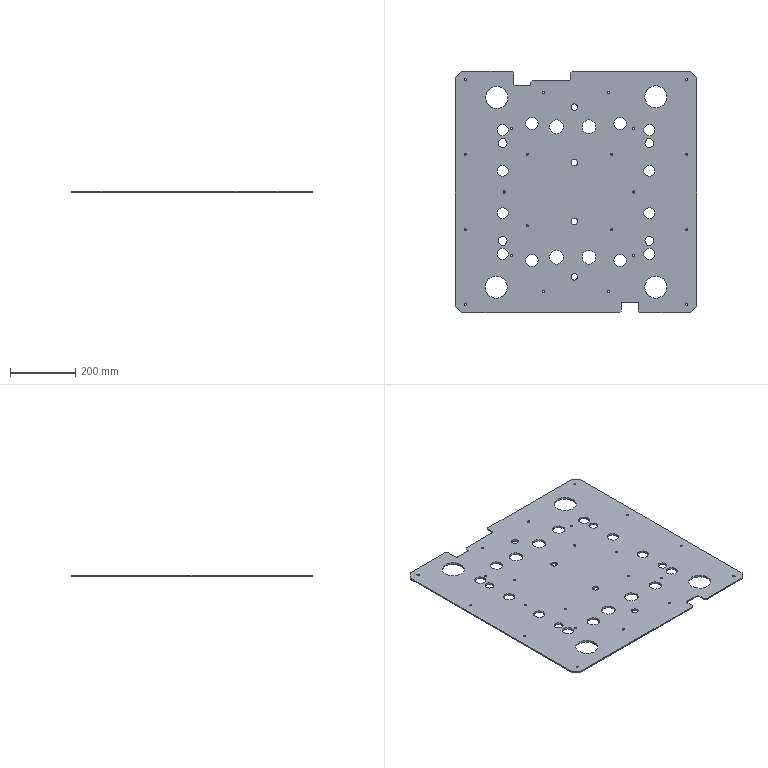Part | Creo | 1 solid | 246 faces | box 740 x 740 x 6 mm | volume 2999442 mm3 | cylinder 149 | cone 49 | plane 48 | commonest cylinder face diameters 6.6 x44 13 x44 34 x16 20 x8 27 x8 38 x8